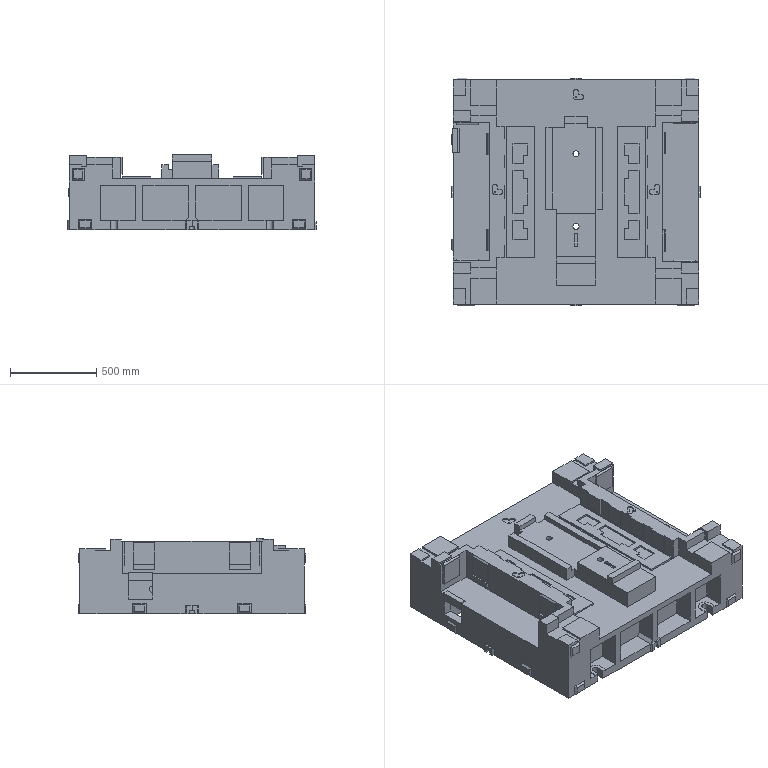Part | NX | features solid 2 | 1 solid | 889 faces | box 1440 x 1320 x 435 mm | volume 308227953 mm3 | plane 737 | cylinder 149 | cone 3 | commonest cylinder face diameters 50 x116 30 x9 10 x6 20 x6 40 x4 80 x4